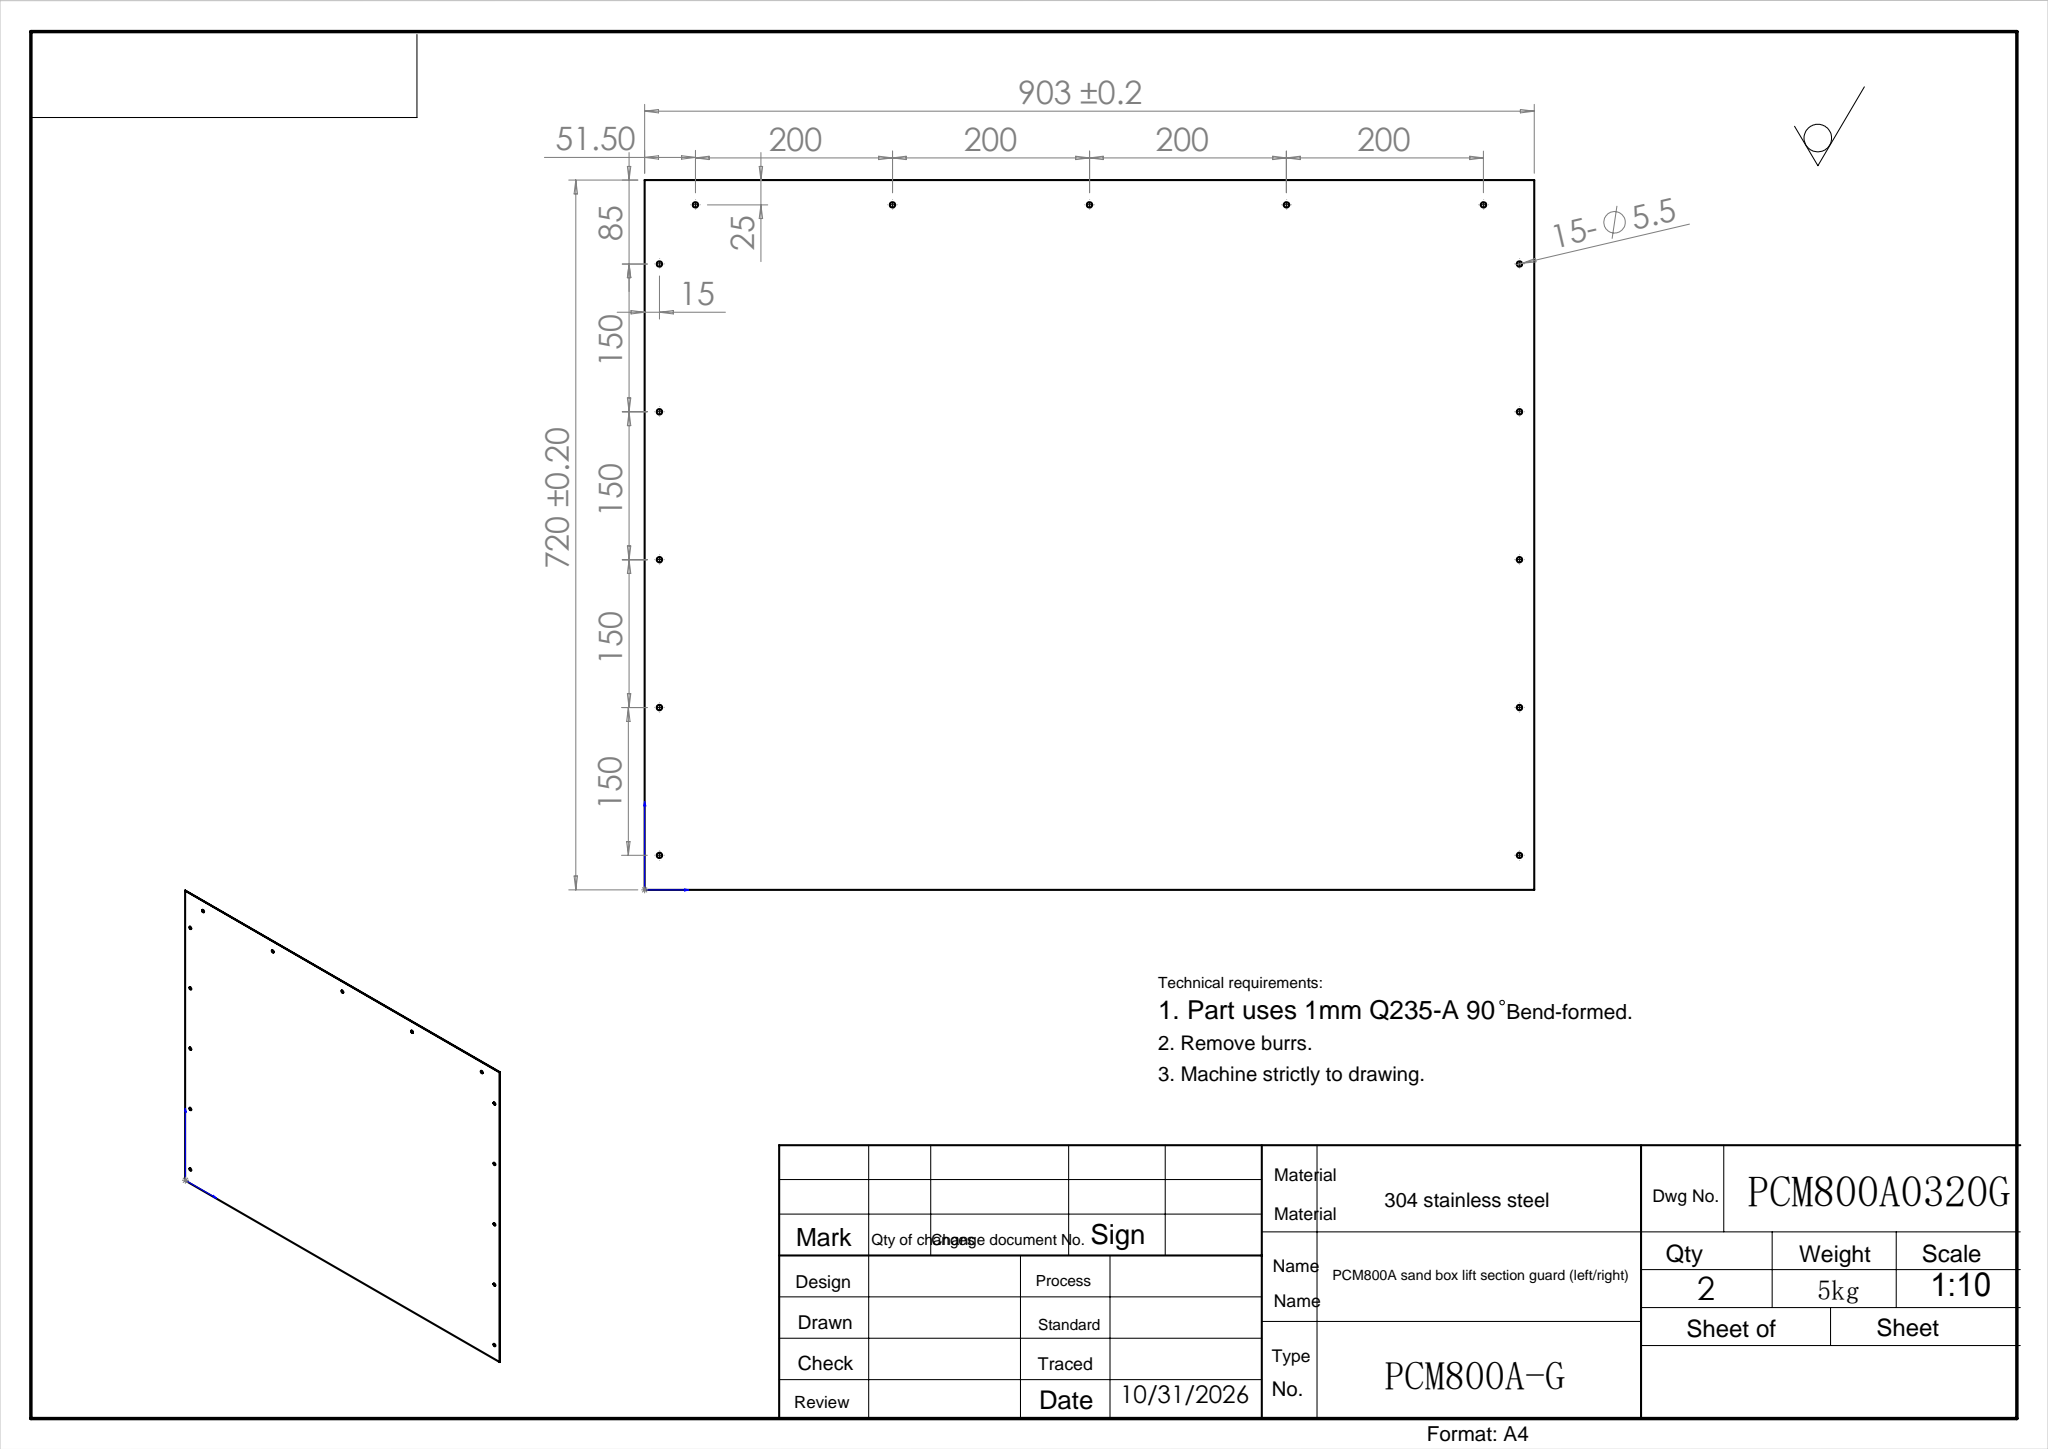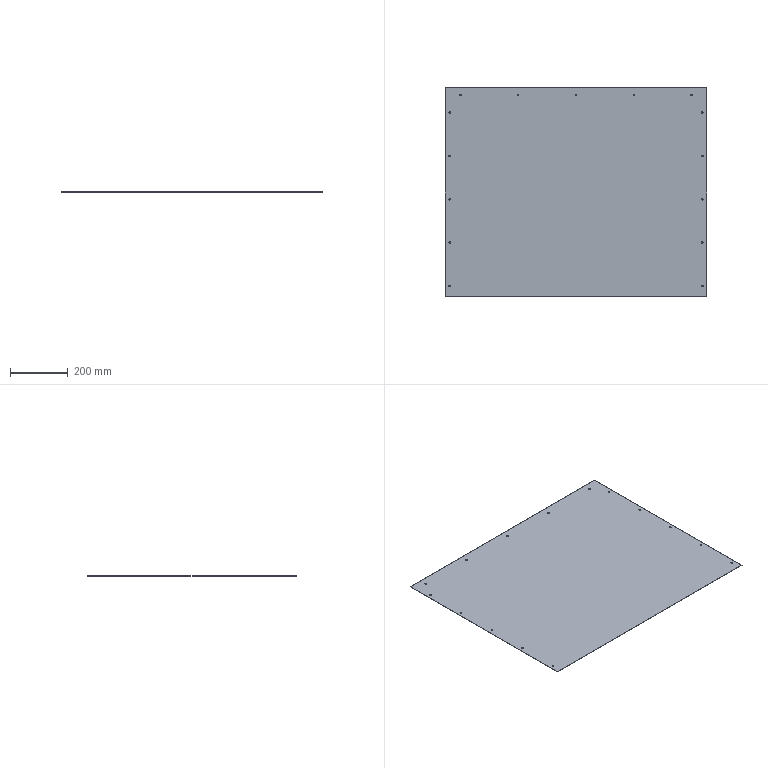Part | SolidWorks | features Extrusion 1, ICE 1 | 1 solid | 36 faces | box 903 x 720 x 1 mm | volume 649804 mm3 | cylinder 30 | plane 6 | commonest cylinder face diameters 5.5 x30